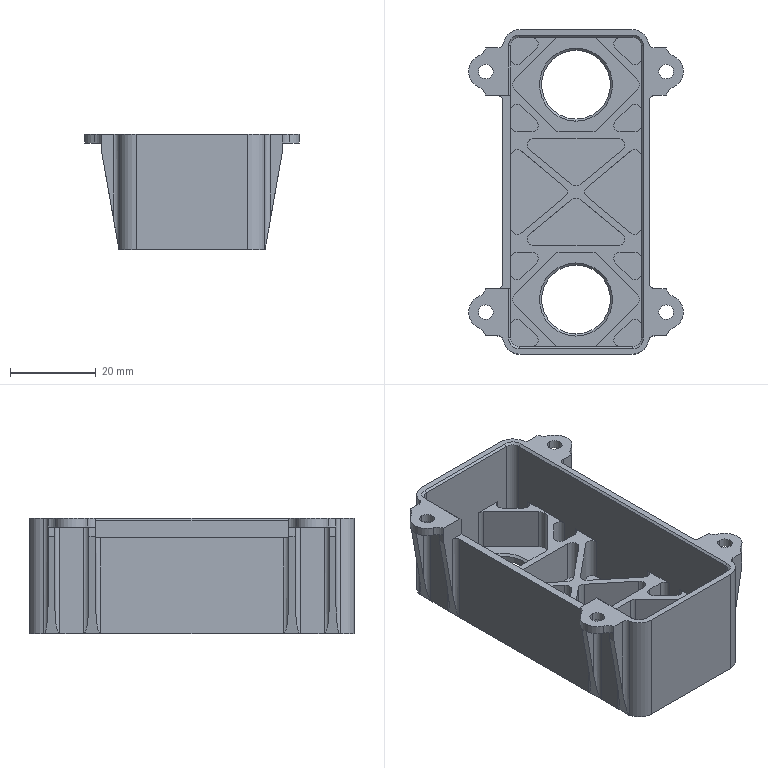NC program | NX | posted with a generic post | part box 50 x 75.58 x 26.8 mm
Lines 19 to 907 of 37241:
(ZLEVEL_PROFILE_COPY , TOOL : D10)
N36 T15 M6
N38 G54
N40 G17 G0 G90 X-44.182 Y16.56 S9500 M3
N42 G43 Z30. H15
N44 Z1.5
N46 G94 G1 X-43.7 Y17.843 Z1.428 F1000.
N48 X-42.604 Y19.631 Z1.318
N50 X-41.19 Y21.179 Z1.208
N52 X-39.509 Y22.432 Z1.099
N54 X-37.62 Y23.344 Z0.989
N56 X-36.839 Y23.569 Z0.946
N58 X-36.251 Y23.833 Z0.912
N60 X-34.626 Y24.179 Z0.825
N62 X-33.98 Y24.177 Z0.791
N64 X-31.421 Z0.657
N66 X-30.813 Y24.192 Z0.625
N68 X-30.384 Y24.145 Z0.603
N70 X-29.794 Y24. Z0.571
N72 X-26.202 Z0.383
N74 X-25.589 Y24.145 Z0.35
N76 X-25.239 Y24.184 Z0.331
N78 X-24.61 Y24.177 Z0.298
N80 X-21.172 Z0.118
N82 X-20.905 Y24.145 Z0.104
N84 X-20.307 Y24. Z0.072
N86 X0. Z-0.993
N88 X20.307 F3200.
N90 G2 X21.89 Y24.177 R6.356
N92 G1 X24.61
N94 G2 X26.285 Y24. R8.667
N96 G1 X29.794
N98 G2 X31.39 Y24.177 R6.066
N100 G1 X33.98
N102 G2 X36.85 Y23.566 R6.905
N104 X44.79 Y13. R11.
N106 G1 Y-13.
N108 G2 X37.1 Y-23.49 R11.
N110 G1 X36.365 Y-23.77
N112 G2 X33.98 Y-24.177 R7.244
N114 G1 X31.39
N116 G2 X29.6 Y-24. R12.175
N118 G1 X26.29
N120 G2 X24.61 Y-24.177 R10.857
N122 G1 X21.89
N124 G2 X20.364 Y-24. R6.047
N126 G1 X-20.209
N128 G2 X-21.89 Y-24.177 R11.324
N130 G1 X-24.61
N132 G2 X-26.124 Y-24. R5.612
N134 G1 X-29.6
N136 G2 X-31.39 Y-24.177 R14.403
N138 G1 X-33.98
N140 G2 X-36.842 Y-23.568 R6.86
N142 X-44.79 Y-13. R11.
N144 G1 Y13.
N146 G2 X-36.839 Y23.569 R11.
N148 X-33.98 Y24.177 R6.925
N150 G1 X-31.421
N152 G2 X-29.794 Y24. R6.136
N154 G1 X-26.202
N156 G2 X-24.61 Y24.177 R6.587
N158 G1 X-21.788
N160 G2 X-20.307 Y24. R6.3
N162 G1 X0.
N164 X19.858 Z-1.339
N166 X20.082 Z-1.343
N168 X20.303 Y24.039 Z-1.347
N170 X20.522 Y24.094 Z-1.351
N172 X20.742 Y24.146 Z-1.355
N174 X21.193 Y24.206 Z-1.363
N176 X21.648 Y24.235 Z-1.371
N178 X22.1 Y24.245 Z-1.379
N180 X22.552 Y24.246 Z-1.386
N182 X24.357 Y24.252 Z-1.418
N184 X24.811 Y24.246 Z-1.426
N186 X25.264 Y24.212 Z-1.434
N188 X25.715 Y24.158 Z-1.442
N190 X26.16 Y24.066 Z-1.45
N192 X26.27 Y24.033 Z-1.451
N194 X26.379 Y24. Z-1.453
N196 X27.053 Z-1.465
N198 X29.31 Z-1.505
N200 X29.761 Y24.051 Z-1.513
N202 X30.201 Y24.153 Z-1.52
N204 X30.642 Y24.225 Z-1.528
N206 X31.097 Y24.257 Z-1.536
N208 X31.552 Y24.274 Z-1.544
N210 X33.357 Y24.279 Z-1.576
N212 X33.81 Y24.281 Z-1.583
N214 X34.263 Y24.271 Z-1.591
N216 X34.719 Y24.231 Z-1.599
N218 X35.173 Y24.176 Z-1.607
N220 X35.615 Y24.063 Z-1.615
N222 X36.054 Y23.935 Z-1.623
N224 X36.477 Y23.781 Z-1.631
N226 X36.894 Y23.607 Z-1.639
N228 X37.309 Y23.422 Z-1.646
N230 X37.734 Y23.269 Z-1.654
N232 X38.152 Y23.098 Z-1.662
N234 X38.563 Y22.911 Z-1.67
N236 X38.965 Y22.707 Z-1.678
N238 X39.359 Y22.486 Z-1.686
N240 X39.743 Y22.25 Z-1.694
N242 X40.118 Y21.998 Z-1.702
N244 X40.482 Y21.731 Z-1.709
N246 X40.834 Y21.449 Z-1.717
N248 X41.175 Y21.153 Z-1.725
N250 X41.503 Y20.843 Z-1.733
N252 X41.818 Y20.52 Z-1.741
N254 X42.12 Y20.184 Z-1.749
N256 X42.407 Y19.837 Z-1.757
N258 X42.681 Y19.478 Z-1.765
N260 X42.939 Y19.107 Z-1.772
N262 X43.182 Y18.727 Z-1.78
N264 X43.409 Y18.337 Z-1.788
N266 X43.619 Y17.938 Z-1.796
N268 X43.814 Y17.531 Z-1.804
N270 X43.991 Y17.116 Z-1.812
N272 X44.151 Y16.694 Z-1.82
N274 X44.294 Y16.266 Z-1.828
N276 X44.419 Y15.832 Z-1.836
N278 X44.526 Y15.394 Z-1.843
N280 X44.616 Y14.951 Z-1.851
N282 X44.686 Y14.506 Z-1.859
N284 X44.739 Y14.057 Z-1.867
N286 X44.773 Y13.607 Z-1.875
N288 X44.789 Y13.157 Z-1.883
N290 X44.79 Y12.705 Z-1.891
N292 Y7.289 Z-1.985
N294 Y-13.
N296 G2 X37.198 Y-23.459 R11.
N298 X33.797 Y-24.352 R6.64
N300 G1 X31.62
N302 G2 X29.464 Y-24. R6.225
N304 G1 X26.713
N306 X25.856 Y-24.195
N308 G2 X24.38 Y-24.352 R6.931
N310 G1 X22.12
N312 G2 X19.94 Y-24. R6.523
N314 G1 X-19.946
N316 G2 X-22.12 Y-24.352 R6.54
N318 G1 X-24.38
N320 G2 X-26.586 Y-24. R6.782
N322 G1 X-29.464
N324 G2 X-31.62 Y-24.352 R6.442
N326 G1 X-33.797
N328 G2 X-37.213 Y-23.454 R6.641
N330 X-44.79 Y-13. R11.
N332 G1 Y13.
N334 G2 X-37.284 Y23.43 R11.
N336 X-33.797 Y24.352 R6.97
N338 G1 X-31.62
N340 G2 X-29.419 Y24. R6.235
N342 G1 X-26.646
N344 G2 X-24.38 Y24.352 R7.185
N346 G1 X-22.227
N348 G2 X-21.32 Y24.318 R12.214
N350 X-19.915 Y24. R5.64
N352 G1 X0.
N354 X19.407 Z-2.324
N356 X19.858 Y24.02 Z-2.332
N358 X20.287 Y24.164 Z-2.34
N360 X20.721 Y24.266 Z-2.348
N362 X21.167 Y24.359 Z-2.355
N364 X21.62 Y24.402 Z-2.363
N366 X22.073 Y24.418 Z-2.371
N368 X22.526 Y24.421 Z-2.379
N370 X23.88 Y24.425 Z-2.403
N372 X24.331 Y24.427 Z-2.411
N374 X24.786 Y24.411 Z-2.418
N376 X25.239 Y24.374 Z-2.426
N378 X25.688 Y24.3 Z-2.434
N380 X26.132 Y24.197 Z-2.442
N382 X26.348 Y24.138 Z-2.446
N384 X26.563 Y24.065 Z-2.45
N386 X26.67 Y24.026 Z-2.452
N388 X26.778 Y24. Z-2.454
N390 X27.002 Z-2.458
N392 X28.807 Z-2.489
N394 X29.253 Z-2.497
N396 X29.464 Y24.082 Z-2.501
N398 X29.677 Y24.151 Z-2.505
N400 X30.118 Y24.271 Z-2.513
N402 X30.564 Y24.366 Z-2.521
N404 X31.018 Y24.417 Z-2.529
N406 X31.475 Y24.445 Z-2.537
N408 X31.926 Y24.45 Z-2.545
N410 X32.378 Y24.452 Z-2.552
N412 X33.28 Y24.454 Z-2.568
N414 X33.734 Y24.456 Z-2.576
N416 X34.188 Y24.441 Z-2.584
N418 X34.643 Y24.397 Z-2.592
N420 X35.097 Y24.338 Z-2.6
N422 X35.538 Y24.22 Z-2.608
N424 X35.976 Y24.088 Z-2.615
N426 X36.403 Y23.928 Z-2.623
N428 X36.824 Y23.753 Z-2.631
N430 X37.22 Y23.539 Z-2.639
N432 X37.612 Y23.315 Z-2.647
N434 X38.032 Y23.149 Z-2.655
N436 X38.445 Y22.967 Z-2.663
N438 X38.85 Y22.767 Z-2.671
N440 X39.246 Y22.552 Z-2.678
N442 X39.633 Y22.32 Z-2.686
N444 X40.011 Y22.072 Z-2.694
N446 X40.377 Y21.809 Z-2.702
N448 X40.733 Y21.532 Z-2.71
N450 X41.077 Y21.24 Z-2.718
N452 X41.409 Y20.934 Z-2.726
N454 X41.728 Y20.615 Z-2.734
N456 X42.034 Y20.283 Z-2.741
N458 X42.326 Y19.938 Z-2.749
N460 X42.603 Y19.583 Z-2.757
N462 X42.866 Y19.216 Z-2.765
N464 X43.113 Y18.838 Z-2.773
N466 X43.345 Y18.451 Z-2.781
N468 X43.56 Y18.054 Z-2.789
N470 X43.759 Y17.649 Z-2.797
N472 X43.941 Y17.236 Z-2.804
N474 X44.107 Y16.816 Z-2.812
N476 X44.255 Y16.39 Z-2.82
N478 X44.385 Y15.958 Z-2.828
N480 X44.497 Y15.521 Z-2.836
N482 X44.592 Y15.08 Z-2.844
N484 X44.668 Y14.635 Z-2.852
N486 X44.726 Y14.187 Z-2.86
N488 X44.765 Y13.738 Z-2.867
N490 X44.786 Y13.287 Z-2.875
N492 X44.79 Y12.836 Z-2.883
N494 Y7.42 Z-2.978
N496 Y-13.
N498 G2 X37.596 Y-23.321 R11.
N500 X33.673 Y-24.527 R6.844
N502 G1 X31.769
N504 G2 X29.119 Y-24. R6.458
N506 G1 X26.863
N508 G2 X24.231 Y-24.527 R6.572
N510 G1 X22.269
N512 G2 X19.627 Y-24. R6.31
N514 G1 X-19.623
N516 G2 X-22.269 Y-24.527 R6.778
N518 G1 X-24.301
N520 G2 X-26.586 Y-24.121 R6.633
N522 G1 X-26.764 Y-24.055
N524 X-26.863 Y-24.
N526 X-29.119
N528 G2 X-31.769 Y-24.527 R6.754
N530 G1 X-33.673
N532 G2 X-36.743 Y-23.819 R6.817
N534 G1 X-36.935 Y-23.73
N536 G2 X-37.559 Y-23.334 R2.524
N538 X-44.79 Y-13. R11.
N540 G1 Y13.
N542 G2 X-37.628 Y23.309 R11.
N544 X-33.673 Y24.527 R6.937
N546 G1 X-31.769
N548 G2 X-29.085 Y24. R6.8
N550 G1 X-26.918
N552 G2 X-24.231 Y24.527 R6.701
N554 G1 X-22.333
N556 G2 X-21.32 Y24.476 R10.159
N558 X-19.609 Y24. R5.868
N560 G1 X0.
N562 X18.955 Z-3.309
N564 X19.402 Z-3.317
N566 X19.615 Y24.052 Z-3.32
N568 X19.821 Y24.15 Z-3.324
N570 X20.253 Y24.289 Z-3.332
N572 X20.693 Y24.403 Z-3.34
N574 X21.139 Y24.493 Z-3.348
N576 X21.587 Y24.569 Z-3.356
N578 X22.041 Y24.589 Z-3.364
N580 X22.495 Y24.596 Z-3.372
N582 X23.397 Y24.599 Z-3.387
N584 X23.848 Y24.6 Z-3.395
N586 X24.3 Y24.601 Z-3.403
N588 X24.755 Y24.582 Z-3.411
N590 X25.209 Y24.535 Z-3.419
N592 X25.656 Y24.449 Z-3.427
N594 X26.098 Y24.34 Z-3.435
N596 X26.52 Y24.215 Z-3.443
N598 X26.937 Y24.049 Z-3.45
N600 X27.06 Y24. Z-3.453
N602 X27.84 Z-3.466
N604 X28.742 Z-3.482
N606 X29.171 Y24.101 Z-3.49
N608 X29.59 Y24.255 Z-3.498
N610 X30.027 Y24.389 Z-3.506
N612 X30.469 Y24.503 Z-3.513
N614 X30.92 Y24.574 Z-3.521
N616 X31.376 Y24.609 Z-3.529
N618 X31.829 Y24.625 Z-3.537
N620 X32.283 Y24.627 Z-3.545
N622 X33.186 Y24.629 Z-3.561
N624 X33.64 Y24.631 Z-3.569
N626 X34.094 Y24.616 Z-3.576
N628 X34.551 Y24.583 Z-3.584
N630 X35.002 Y24.509 Z-3.592
N632 X35.445 Y24.394 Z-3.6
N634 X35.884 Y24.265 Z-3.608
N636 X36.31 Y24.102 Z-3.616
N638 X36.726 Y23.914 Z-3.624
N640 X37.135 Y23.713 Z-3.632
N642 X37.519 Y23.466 Z-3.64
N644 X37.701 Y23.334 Z-3.643
N646 X37.887 Y23.209 Z-3.647
N648 X38.094 Y23.123 Z-3.651
N650 X38.299 Y23.033 Z-3.655
N652 X38.707 Y22.84 Z-3.663
N654 X39.107 Y22.63 Z-3.671
N656 X39.497 Y22.404 Z-3.679
N658 X39.878 Y22.162 Z-3.687
N660 X40.249 Y21.904 Z-3.695
N662 X40.608 Y21.632 Z-3.703
N664 X40.957 Y21.345 Z-3.71
N666 X41.293 Y21.044 Z-3.718
N668 X41.617 Y20.729 Z-3.726
N670 X41.927 Y20.402 Z-3.734
N672 X42.224 Y20.062 Z-3.742
N674 X42.506 Y19.71 Z-3.75
N676 X42.774 Y19.347 Z-3.758
N678 X43.027 Y18.973 Z-3.766
N680 X43.264 Y18.589 Z-3.773
N682 X43.486 Y18.196 Z-3.781
N684 X43.691 Y17.794 Z-3.789
N686 X43.879 Y17.384 Z-3.797
N688 X44.05 Y16.966 Z-3.805
N690 X44.204 Y16.542 Z-3.813
N692 X44.341 Y16.112 Z-3.821
N694 X44.459 Y15.676 Z-3.829
N696 X44.56 Y15.236 Z-3.836
N698 X44.643 Y14.793 Z-3.844
N700 X44.707 Y14.346 Z-3.852
N702 X44.753 Y13.897 Z-3.86
N704 X44.781 Y13.447 Z-3.868
N706 X44.79 Y12.996 Z-3.876
N708 Y7.58 Z-3.97
N710 Y-13.
N712 G2 X37.917 Y-23.196 R11.
N714 X33.588 Y-24.702 R6.86
N716 G1 X31.872
N718 G2 X28.835 Y-24. R6.487
N720 G1 X27.17
N722 G2 X24.128 Y-24.702 R6.797
N724 G1 X22.372
N726 G2 X19.33 Y-24. R6.701
N728 G1 X-19.33
N730 G2 X-22.372 Y-24.702 R6.814
N732 G1 X-24.128
N734 G2 X-27.184 Y-24. R6.824
N736 G1 X-28.836
N738 G2 X-31.872 Y-24.702 R6.742
N740 G1 X-33.588
N742 G2 X-37.916 Y-23.197 R6.832
N744 X-44.79 Y-13. R11.
N746 G1 Y13.
N748 G2 X-37.988 Y23.167 R11.
N750 X-33.588 Y24.702 R7.083
N752 G1 X-31.872
N754 G2 X-28.786 Y24. R7.094
N756 G1 X-27.228
N758 G2 X-24.128 Y24.702 R7.211
N760 G1 X-22.345
N762 G2 X-19.837 Y24.243 R7.089
N764 G1 X-19.31 Y24.
N766 X0.
N768 X18.955 Z-4.301
N770 X19.177 Z-4.305
N772 X19.281 Y24.033 Z-4.307
N774 X19.382 Y24.084 Z-4.309
N776 X19.584 Y24.18 Z-4.313
N778 X19.786 Y24.285 Z-4.317
N780 X20.22 Y24.419 Z-4.325
N782 X20.656 Y24.549 Z-4.333
N784 X21.101 Y24.645 Z-4.341
N786 X21.548 Y24.735 Z-4.349
N788 X22.002 Y24.76 Z-4.356
N790 X22.457 Y24.771 Z-4.364
N792 X23.36 Y24.774 Z-4.38
N794 X23.812 Y24.775 Z-4.388
N796 X24.264 Z-4.396
N798 X24.719 Y24.75 Z-4.404
N800 X25.172 Y24.7 Z-4.412
N802 X25.619 Y24.612 Z-4.419
N804 X26.062 Y24.505 Z-4.427
N806 X26.494 Y24.364 Z-4.435
N808 X26.917 Y24.195 Z-4.443
N810 X27.406 Y24. Z-4.452
N812 X27.768 Z-4.459
N814 X28.671 Z-4.475
N816 X29.077 Y24.202 Z-4.482
N818 X29.491 Y24.363 Z-4.49
N820 X29.924 Y24.506 Z-4.498
N822 X30.364 Y24.627 Z-4.506
N824 X30.813 Y24.71 Z-4.514
N826 X31.266 Y24.769 Z-4.522
N828 X31.72 Y24.798 Z-4.53
N830 X32.175 Y24.802 Z-4.538
N832 X33.078 Y24.804 Z-4.553
N834 X33.532 Y24.806 Z-4.561
N836 X33.986 Y24.794 Z-4.569
N838 X34.442 Y24.752 Z-4.577
N840 X34.895 Y24.687 Z-4.585
N842 X35.34 Y24.579 Z-4.593
N844 X35.78 Y24.455 Z-4.601
N846 X36.207 Y24.291 Z-4.608
N848 X36.627 Y24.111 Z-4.616
N850 X37.028 Y23.895 Z-4.624
N852 X37.419 Y23.659 Z-4.632
N854 X37.789 Y23.407 Z-4.64
N856 X38.134 Y23.109 Z-4.648
N858 X38.544 Y22.92 Z-4.656
N860 X38.947 Y22.716 Z-4.664
N862 X39.341 Y22.497 Z-4.671
N864 X39.726 Y22.261 Z-4.679
N866 X40.101 Y22.01 Z-4.687
N868 X40.465 Y21.743 Z-4.695
N870 X40.818 Y21.462 Z-4.703
N872 X41.159 Y21.167 Z-4.711
N874 X41.488 Y20.858 Z-4.719
N876 X41.804 Y20.535 Z-4.727
N878 X42.106 Y20.2 Z-4.735
N880 X42.394 Y19.853 Z-4.742
N882 X42.668 Y19.494 Z-4.75
N884 X42.927 Y19.125 Z-4.758
N886 X43.171 Y18.745 Z-4.766
N888 X43.398 Y18.355 Z-4.774
N890 X43.61 Y17.957 Z-4.782
N892 X43.805 Y17.55 Z-4.79
N894 X43.983 Y17.135 Z-4.798
N896 X44.144 Y16.713 Z-4.805
N898 X44.288 Y16.286 Z-4.813
N900 X44.414 Y15.852 Z-4.821
N902 X44.522 Y15.414 Z-4.829
N904 X44.612 Y14.972 Z-4.837
N906 X44.684 Y14.526 Z-4.845
N908 X44.737 Y14.078 Z-4.853
N910 X44.772 Y13.628 Z-4.861
N912 X44.789 Y13.177 Z-4.868
N914 X44.79 Y12.726 Z-4.876
N916 Y12.275 Z-4.884
N918 Y7.762 Z-4.963
N920 Y-13.
N922 G2 X38.258 Y-23.052 R11.
N924 X33.534 Y-24.877 R7.042
N926 G1 X31.943
N928 G2 X28.562 Y-24. R6.729
N930 G1 X27.446
N932 G2 X24.057 Y-24.877 R6.88
N934 G1 X22.443
N936 G2 X19.069 Y-24. R6.482
N938 G1 X-19.037
N940 G2 X-22.443 Y-24.877 R7.022
N942 G1 X-24.057
N944 G2 X-27.447 Y-24. R6.778
N946 G1 X-28.562
N948 G2 X-31.943 Y-24.877 R6.791
N950 G1 X-33.534
N952 G2 X-38.248 Y-23.056 R6.999
N954 X-44.79 Y-13. R11.
N956 G1 Y13.
N958 G2 X-38.213 Y23.072 R11.
N960 G1 X-38.067 Y23.227
N962 X-37.565 Y23.59
N964 G2 X-33.594 Y24.877 R6.773
N966 G1 X-31.943
N968 G2 X-28.549 Y24. R6.813
N970 G1 X-27.476
N972 G2 X-24.057 Y24.877 R7.042
N974 G1 X-22.443
N976 G2 X-19.031 Y24. R6.99
N978 G1 X0.
N980 X18.955 Z-5.294
N982 X19.354 Y24.219 Z-5.302
N984 X19.76 Y24.401 Z-5.31
N986 X20.186 Y24.56 Z-5.317
N988 X20.618 Y24.699 Z-5.325
N990 X20.84 Y24.752 Z-5.329
N992 X21.058 Y24.82 Z-5.333
N994 X21.283 Y24.858 Z-5.337
N996 X21.51 Y24.881 Z-5.341
N998 X21.963 Y24.932 Z-5.349
N1000 X22.418 Y24.946 Z-5.357
N1002 X22.87 Y24.947 Z-5.365
N1004 X23.321 Y24.949 Z-5.373
N1006 X23.773 Y24.95 Z-5.38
N1008 X24.225 Y24.949 Z-5.388
N1010 X24.68 Y24.924 Z-5.396
N1012 X25.133 Y24.868 Z-5.404
N1014 X25.581 Y24.784 Z-5.412
N1016 X26.023 Y24.675 Z-5.42
N1018 X26.454 Y24.528 Z-5.428
N1020 X26.877 Y24.358 Z-5.436
N1022 X27.279 Y24.173 Z-5.444
N1024 X27.684 Y24. Z-5.451
N1026 X28.217 Z-5.461
N1028 X28.548 Y24.08 Z-5.467
N1030 X28.952 Y24.293 Z-5.475
N1032 X29.37 Y24.475 Z-5.483
N1034 X29.8 Y24.626 Z-5.491
N1036 X30.237 Y24.758 Z-5.499
N1038 X30.684 Y24.854 Z-5.507
N1040 X31.135 Y24.924 Z-5.514
N1042 X31.59 Y24.965 Z-5.522
N1044 X32.046 Y24.977 Z-5.53
N1046 X32.949 Y24.979 Z-5.546
N1048 X33.402 Y24.981 Z-5.554
N1050 X33.856 Y24.974 Z-5.562
N1052 X34.312 Y24.938 Z-5.57
N1054 X34.766 Y24.874 Z-5.577
N1056 X35.213 Y24.777 Z-5.585
N1058 X35.655 Y24.657 Z-5.593
N1060 X36.084 Y24.5 Z-5.601
N1062 X36.505 Y24.319 Z-5.609
N1064 X36.912 Y24.111 Z-5.617
N1066 X37.306 Y23.879 Z-5.625
N1068 X37.683 Y23.621 Z-5.633
N1070 X38.045 Y23.343 Z-5.64
N1072 X38.209 Y23.19 Z-5.644
N1074 X38.372 Y23.035 Z-5.648
N1076 X38.556 Y22.914 Z-5.652
N1078 X38.756 Y22.815 Z-5.656
N1080 X39.155 Y22.603 Z-5.664
N1082 X39.544 Y22.375 Z-5.672
N1084 X39.924 Y22.131 Z-5.68
N1086 X40.293 Y21.872 Z-5.688
N1088 X40.651 Y21.598 Z-5.696
N1090 X40.998 Y21.309 Z-5.703
N1092 X41.333 Y21.006 Z-5.711
N1094 X41.655 Y20.69 Z-5.719
N1096 X41.964 Y20.361 Z-5.727
N1098 X42.259 Y20.02 Z-5.735
N1100 X42.54 Y19.666 Z-5.743
N1102 X42.806 Y19.302 Z-5.751
N1104 X43.057 Y18.927 Z-5.759
N1106 X43.292 Y18.542 Z-5.766
N1108 X43.511 Y18.147 Z-5.774
N1110 X43.714 Y17.744 Z-5.782
N1112 X43.901 Y17.333 Z-5.79
N1114 X44.07 Y16.915 Z-5.798
N1116 X44.222 Y16.49 Z-5.806
N1118 X44.356 Y16.059 Z-5.814
N1120 X44.473 Y15.623 Z-5.822
N1122 X44.571 Y15.183 Z-5.83
N1124 X44.652 Y14.739 Z-5.837
N1126 X44.714 Y14.292 Z-5.845
N1128 X44.758 Y13.842 Z-5.853
N1130 X44.783 Y13.392 Z-5.861
N1132 X44.79 Y12.941 Z-5.869
N1134 Y12.489 Z-5.877
N1136 Y7.976 Z-5.956
N1138 Y-13.
N1140 G2 X38.537 Y-22.923 R11.
N1142 X33.505 Y-25.052 R7.023
N1144 G1 X31.983
N1146 G2 X28.292 Y-24. R6.971
N1148 G1 X27.708
N1150 G2 X24.017 Y-25.052 R6.964
N1152 G1 X22.483
N1154 G2 X18.792 Y-24. R6.955
N1156 G1 X-18.787
N1158 G2 X-22.483 Y-25.052 R7.013
N1160 G1 X-24.017
N1162 G2 X-27.708 Y-24. R6.951
N1164 G1 X-28.292
N1166 G2 X-31.983 Y-25.052 R6.993
N1168 G1 X-33.505
N1170 G2 X-38.513 Y-22.934 R6.947
N1172 X-44.79 Y-13. R11.
N1174 G1 Y13.
N1176 G2 X-38.523 Y22.93 R11.
N1178 X-33.505 Y25.052 R6.822
N1180 G1 X-31.983
N1182 G2 X-28.302 Y24. R6.876
N1184 G1 X-27.71
N1186 G2 X-24.017 Y25.052 R6.889
N1188 G1 X-22.483
N1190 G2 X-18.809 Y24. R6.826
N1192 G1 X0.
N1194 X18.053 Z-6.271
N1196 X18.641 Z-6.281
N1198 X18.906 Y24.135 Z-6.286
N1200 X19.306 Y24.351 Z-6.294
N1202 X19.716 Y24.546 Z-6.302
N1204 X20.141 Y24.708 Z-6.31
N1206 X20.573 Y24.851 Z-6.318
N1208 X21.012 Y24.974 Z-6.326
N1210 X21.462 Y25.043 Z-6.334
N1212 X21.914 Y25.101 Z-6.342
N1214 X22.369 Y25.121 Z-6.349
N1216 X22.821 Y25.123 Z-6.357
N1218 X23.273 Y25.124 Z-6.365
N1220 X23.725 Y25.125 Z-6.373
N1222 X24.177 Z-6.381
N1224 X24.633 Y25.1 Z-6.389
N1226 X25.086 Y25.046 Z-6.397
N1228 X25.534 Y24.962 Z-6.405
N1230 X25.976 Y24.852 Z-6.412
N1232 X26.409 Y24.708 Z-6.42
N1234 X26.832 Y24.539 Z-6.428
N1236 X27.246 Y24.347 Z-6.436
N1238 X27.642 Y24.122 Z-6.444
N1240 X27.861 Y24. Z-6.448
N1242 X28.121 Z-6.454
N1244 X28.424 Y24.166 Z-6.46
N1246 X28.824 Y24.386 Z-6.468
N1248 X29.238 Y24.578 Z-6.475
N1250 X29.663 Y24.745 Z-6.483
N1252 X30.097 Y24.886 Z-6.491
N1254 X30.541 Y24.995 Z-6.499
N1256 X30.991 Y25.077 Z-6.507
N1258 X31.446 Y25.129 Z-6.515
N1260 X31.903 Y25.151 Z-6.523
N1262 X32.354 Y25.153 Z-6.531
N1264 X32.806 Y25.154 Z-6.539
N1266 X33.259 Y25.156 Z-6.546
N1268 X33.712 Y25.154 Z-6.554
N1270 X34.169 Y25.127 Z-6.562
N1272 X34.624 Y25.069 Z-6.57
N1274 X35.073 Y24.982 Z-6.578
N1276 X35.516 Y24.866 Z-6.586
N1278 X35.951 Y24.721 Z-6.594
N1280 X36.375 Y24.548 Z-6.602
N1282 X36.786 Y24.348 Z-6.609
N1284 X37.183 Y24.121 Z-6.617
N1286 X37.565 Y23.869 Z-6.625
N1288 X37.929 Y23.592 Z-6.633
N1290 X38.261 Y23.304 Z-6.641
N1292 X38.578 Y22.991 Z-6.649
N1294 X38.66 Y22.904 Z-6.651
N1296 X38.744 Y22.821 Z-6.653
N1298 X38.845 Y22.77 Z-6.655
N1300 X38.945 Y22.717 Z-6.657
N1302 X39.144 Y22.609 Z-6.661
N1304 X39.341 Y22.497 Z-6.665
N1306 X39.726 Y22.261 Z-6.672
N1308 X40.101 Y22.01 Z-6.68
N1310 X40.465 Y21.743 Z-6.688
N1312 X40.818 Y21.462 Z-6.696
N1314 X41.159 Y21.167 Z-6.704
N1316 X41.488 Y20.858 Z-6.712
N1318 X41.804 Y20.535 Z-6.72
N1320 X42.106 Y20.2 Z-6.728
N1322 X42.394 Y19.853 Z-6.735
N1324 X42.668 Y19.494 Z-6.743
N1326 X42.927 Y19.125 Z-6.751
N1328 X43.171 Y18.745 Z-6.759
N1330 X43.398 Y18.355 Z-6.767
N1332 X43.61 Y17.957 Z-6.775
N1334 X43.805 Y17.55 Z-6.783
N1336 X43.983 Y17.135 Z-6.791
N1338 X44.144 Y16.713 Z-6.798
N1340 X44.288 Y16.286 Z-6.806
N1342 X44.414 Y15.852 Z-6.814
N1344 X44.522 Y15.414 Z-6.822
N1346 X44.612 Y14.972 Z-6.83
N1348 X44.684 Y14.526 Z-6.838
N1350 X44.737 Y14.078 Z-6.846
N1352 X44.772 Y13.628 Z-6.854
N1354 X44.789 Y13.177 Z-6.861
N1356 X44.79 Y12.726 Z-6.869
N1358 Y8.213 Z-6.948
N1360 Y-13.
N1362 G2 X38.808 Y-22.789 R11.
N1364 X33.5 Y-25.227 R7.004
N1366 G1 X31.999
N1368 G2 X28.03 Y-24. R7.091
N1370 G1 X27.94
N1372 G2 X24.001 Y-25.227 R6.862
N1374 G1 X22.499
N1376 G2 X18.54 Y-24. R7.009
N1378 G1 X-18.54
N1380 G2 X-22.499 Y-25.227 R7.009
N1382 G1 X-24.001
N1384 G2 X-27.949 Y-24. R6.913
N1386 G1 X-28.04
N1388 G2 X-31.999 Y-25.227 R7.013
N1390 G1 X-33.5
N1392 G2 X-38.809 Y-22.788 R6.998
N1394 X-44.79 Y-13. R11.
N1396 G1 Y13.
N1398 G2 X-38.79 Y22.798 R11.
N1400 X-33.5 Y25.227 R6.883
N1402 G1 X-31.999
N1404 G2 X-28.03 Y24. R7.09
N1406 G1 X-27.94
N1408 G2 X-26.105 Y24.9 R5.839
N1410 X-24.001 Y25.227 R6.599
N1412 G1 X-22.499
N1414 G2 X-18.54 Y24. R7.002
N1416 G1 X0.
N1418 X18.053 Z-7.263
N1420 X18.327 Z-7.268
N1422 X18.859 Y24.275 Z-7.279
N1424 X19.259 Y24.491 Z-7.287
N1426 X19.666 Y24.693 Z-7.295
N1428 X20.084 Y24.876 Z-7.303
N1430 X20.52 Y25.006 Z-7.311
N1432 X20.959 Y25.129 Z-7.318
N1434 X21.407 Y25.209 Z-7.326
N1436 X21.859 Y25.269 Z-7.334
N1438 X22.314 Y25.295 Z-7.342
N1440 X22.766 Y25.298 Z-7.35
N1442 X23.218 Y25.299 Z-7.358
N1444 X23.67 Y25.3 Z-7.366
N1446 X24.122 Y25.301 Z-7.374
N1448 X24.577 Y25.279 Z-7.381
N1450 X25.031 Y25.228 Z-7.389
N1452 X25.48 Y25.148 Z-7.397
N1454 X25.922 Y25.038 Z-7.405
N1456 X26.357 Y24.9 Z-7.413
N1458 X26.782 Y24.733 Z-7.421
N1460 X27.195 Y24.539 Z-7.429
N1462 X27.595 Y24.319 Z-7.437
N1464 X28.001 Y24.06 Z-7.446
N1466 X28.289 Y24.251 Z-7.452
N1468 X28.683 Y24.481 Z-7.46
N1470 X29.091 Y24.685 Z-7.468
N1472 X29.512 Y24.863 Z-7.476
N1474 X29.944 Y25.012 Z-7.484
N1476 X30.384 Y25.133 Z-7.492
N1478 X30.832 Y25.226 Z-7.5
N1480 X31.285 Y25.289 Z-7.507
N1482 X31.742 Y25.322 Z-7.515
N1484 X32.195 Y25.328 Z-7.523
N1486 X32.648 Y25.329 Z-7.531
N1488 X33.1 Y25.331 Z-7.539
N1490 X33.551 Y25.332 Z-7.547
N1492 X34.009 Y25.315 Z-7.555
N1494 X34.465 Y25.268 Z-7.563
N1496 X34.916 Y25.192 Z-7.57
N1498 X35.362 Y25.085 Z-7.578
N1500 X35.8 Y24.951 Z-7.586
N1502 X36.228 Y24.787 Z-7.594
N1504 X36.644 Y24.596 Z-7.602
N1506 X37.046 Y24.378 Z-7.61
N1508 X37.434 Y24.134 Z-7.618
N1510 X37.804 Y23.866 Z-7.626
N1512 X38.156 Y23.574 Z-7.634
N1514 X38.488 Y23.259 Z-7.641
N1516 X38.789 Y22.93 Z-7.649
N1518 X39.11 Y22.628 Z-7.657
N1520 X39.501 Y22.401 Z-7.665
N1522 X39.882 Y22.159 Z-7.673
N1524 X40.252 Y21.902 Z-7.681
N1526 X40.612 Y21.629 Z-7.689
N1528 X40.96 Y21.342 Z-7.697
N1530 X41.296 Y21.041 Z-7.704
N1532 X41.62 Y20.726 Z-7.712
N1534 X41.93 Y20.399 Z-7.72
N1536 X42.227 Y20.059 Z-7.728
N1538 X42.509 Y19.707 Z-7.736
N1540 X42.777 Y19.343 Z-7.744
N1542 X43.029 Y18.969 Z-7.752
N1544 X43.266 Y18.585 Z-7.76
N1546 X43.488 Y18.192 Z-7.767
N1548 X43.692 Y17.79 Z-7.775
N1550 X43.881 Y17.38 Z-7.783
N1552 X44.052 Y16.962 Z-7.791
N1554 X44.206 Y16.538 Z-7.799
N1556 X44.342 Y16.108 Z-7.807
N1558 X44.46 Y15.672 Z-7.815
N1560 X44.561 Y15.232 Z-7.823
N1562 X44.644 Y14.789 Z-7.83
N1564 X44.708 Y14.342 Z-7.838
N1566 X44.754 Y13.893 Z-7.846
N1568 X44.781 Y13.443 Z-7.854
N1570 X44.79 Y12.991 Z-7.862
N1572 Y8.478 Z-7.941
N1574 Y-13.
N1576 G2 X39.061 Y-22.655 R11.
N1578 X33.5 Y-25.402 R7.014
N1580 G1 X32.
N1582 G2 X28. Y-24.146 R7.012
N1584 X24. Y-25.402 R7.016
N1586 G1 X22.5
N1588 G2 X18.31 Y-24. R6.921
N1590 G1 X-18.31
N1592 G2 X-22.5 Y-25.402 R6.921
N1594 G1 X-24.
N1596 G2 X-28. Y-24.146 R7.016
N1598 X-32. Y-25.402 R7.01
N1600 G1 X-33.5
N1602 G2 X-39.064 Y-22.653 R7.021
N1604 X-44.79 Y-13. R11.
N1606 G1 Y13.
N1608 G2 X-39.048 Y22.662 R11.
N1610 X-33.5 Y25.402 R6.952
N1612 G1 X-32.
N1614 G2 X-28. Y24.146 R7.
N1616 X-24. Y25.402 R6.97
N1618 G1 X-22.5
N1620 G2 X-18.31 Y24. R6.919
N1622 G1 X0.
N1624 X18.053 Z-8.256
N1626 X18.162 Z-8.258
N1628 X18.263 Y24.03 Z-8.26
N1630 X18.354 Y24.097 Z-8.262
N1632 X18.444 Y24.163 Z-8.264
N1634 X18.627 Y24.292 Z-8.268
N1636 X18.811 Y24.415 Z-8.272
N1638 X19.203 Y24.645 Z-8.279
N1640 X19.614 Y24.841 Z-8.287
N1642 X20.033 Y25.02 Z-8.295
N1644 X20.464 Y25.165 Z-8.303
N1646 X20.904 Y25.286 Z-8.311
N1648 X21.348 Y25.389 Z-8.319
N1650 X21.801 Y25.436 Z-8.327
N1652 X22.256 Y25.469 Z-8.335
N1654 X22.708 Y25.473 Z-8.343
N1656 X23.161 Y25.474 Z-8.35
N1658 X23.612 Y25.475 Z-8.358
N1660 X24.064 Y25.476 Z-8.366
N1662 X24.52 Y25.459 Z-8.374
N1664 X24.973 Y25.411 Z-8.382
N1666 X25.423 Y25.335 Z-8.39
N1668 X25.867 Y25.229 Z-8.398
N1670 X26.303 Y25.094 Z-8.406
N1672 X26.729 Y24.931 Z-8.413
N1674 X27.143 Y24.741 Z-8.421
N1676 X27.545 Y24.524 Z-8.429
N1678 X28.016 Y24.245 Z-8.44
N1680 X28.226 Y24.385 Z-8.445
N1682 X28.617 Y24.62 Z-8.453
N1684 X29.023 Y24.829 Z-8.461
N1686 X29.442 Y25.011 Z-8.469
N1688 X29.872 Y25.165 Z-8.476
N1690 X30.312 Y25.291 Z-8.484
N1692 X30.758 Y25.388 Z-8.492
N1694 X31.211 Y25.456 Z-8.5
N1696 X31.667 Y25.494 Z-8.508
N1698 X32.12 Y25.503 Z-8.516
N1700 X32.574 Y25.505 Z-8.524
N1702 X33.477 Y25.507 Z-8.539
N1704 X33.934 Y25.495 Z-8.547
N1706 X34.39 Y25.453 Z-8.555
N1708 X34.843 Y25.381 Z-8.563
N1710 X35.29 Y25.28 Z-8.571
N1712 X35.729 Y25.15 Z-8.579
N1714 X36.159 Y24.991 Z-8.587
N1716 X36.577 Y24.804 Z-8.595
N1718 X36.982 Y24.59 Z-8.602
N1720 X37.372 Y24.351 Z-8.61
N1722 X37.745 Y24.086 Z-8.618
N1724 X38.1 Y23.798 Z-8.626
N1726 X38.434 Y23.486 Z-8.634
N1728 X38.749 Y23.155 Z-8.642
N1730 X39.036 Y22.8 Z-8.65
N1732 X39.173 Y22.626 Z-8.654
N1734 X39.347 Y22.493 Z-8.658
N1736 X39.538 Y22.379 Z-8.662
N1738 X39.725 Y22.261 Z-8.665
N1740 X40.1 Y22.01 Z-8.673
N1742 X40.464 Y21.744 Z-8.681
N1744 X40.817 Y21.463 Z-8.689
N1746 X41.159 Y21.167 Z-8.697
N1748 X41.487 Y20.858 Z-8.705
N1750 X41.803 Y20.536 Z-8.713
N1752 X42.106 Y20.201 Z-8.721
N1754 X42.394 Y19.854 Z-8.729
N1756 X42.668 Y19.495 Z-8.736
N1758 X42.927 Y19.125 Z-8.744
N1760 X43.17 Y18.745 Z-8.752
N1762 X43.398 Y18.356 Z-8.76
N1764 X43.61 Y17.957 Z-8.768
N1766 X43.805 Y17.55 Z-8.776
N1768 X43.983 Y17.136 Z-8.784
N1770 X44.144 Y16.714 Z-8.792
N1772 X44.288 Y16.286 Z-8.799
N1774 X44.414 Y15.853 Z-8.807
N1776 X44.522 Y15.415 Z-8.815
N1778 X44.612 Y14.973 Z-8.823
N1780 X44.683 Y14.527 Z-8.831
N1782 X44.737 Y14.079 Z-8.839
N1784 X44.772 Y13.629 Z-8.847
N1786 X44.789 Y13.178 Z-8.855
N1788 X44.79 Y12.727 Z-8.862
N1790 Y12.275 Z-8.87
N1792 Y8.665 Z-8.933
N1794 Y-13.
N1796 G2 X39.263 Y-22.542 R11.
N1798 X33.5 Y-25.577 R6.983
N1800 G1 X32.
N1802 G2 X28. Y-24.321 R7.
N1804 X24. Y-25.577 R7.02
N1806 G1 X22.5